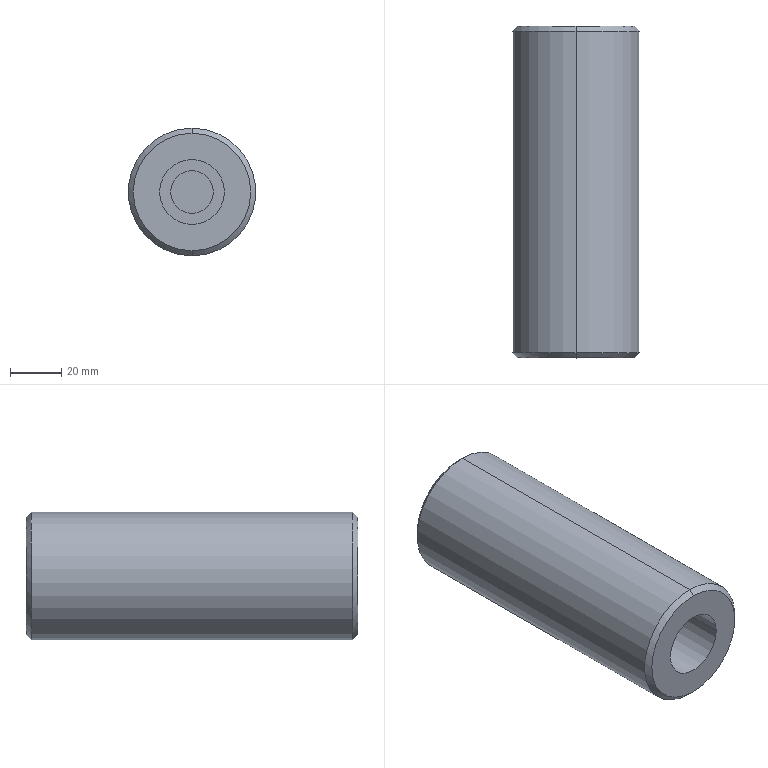Part | STEP file | 4-20.sldasm-Part-91 | 1 solid | 14 faces | box 50 x 130 x 50 mm | volume 218247 mm3 | cylinder 6 | cone 4 | plane 4 | commonest cylinder face diameters 16.667 x2 25.4 x2 50 x2
STEP:
#1=CARTESIAN_POINT('',(131.666,-614.601,200.));
#2=VERTEX_POINT('',#1);
#3=CARTESIAN_POINT('',(148.334,-614.601,200.));
#4=VERTEX_POINT('',#3);
#5=CARTESIAN_POINT('',(140.,-614.601,200.));
#6=DIRECTION('',(0.,-1.,0.));
#7=DIRECTION('',(0.,0.,-1.));
#8=AXIS2_PLACEMENT_3D('',#5,#6,#7);
#9=CIRCLE('',#8,8.334);
#10=EDGE_CURVE('',#2,#4,#9,.T.);
#11=ORIENTED_EDGE('',*,*,#10,.T.);
#12=CARTESIAN_POINT('',(148.334,-530.,200.));
#13=VERTEX_POINT('',#12);
#14=CARTESIAN_POINT('',(148.334,-632.601,200.));
#15=DIRECTION('',(0.,1.,0.));
#16=VECTOR('',#15,1000.);
#17=LINE('',#14,#16);
#18=EDGE_CURVE('',#4,#13,#17,.T.);
#19=ORIENTED_EDGE('',*,*,#18,.T.);
#20=CARTESIAN_POINT('',(131.666,-530.,200.));
#21=VERTEX_POINT('',#20);
#22=CARTESIAN_POINT('',(140.,-530.,200.));
#23=DIRECTION('',(0.,-1.,0.));
#24=DIRECTION('',(0.,0.,-1.));
#25=AXIS2_PLACEMENT_3D('',#22,#23,#24);
#26=CIRCLE('',#25,8.334);
#27=EDGE_CURVE('',#21,#13,#26,.T.);
#28=ORIENTED_EDGE('',*,*,#27,.F.);
#29=CARTESIAN_POINT('',(131.666,-632.601,200.));
#30=DIRECTION('',(0.,1.,0.));
#31=VECTOR('',#30,1000.);
#32=LINE('',#29,#31);
#33=EDGE_CURVE('',#2,#21,#32,.T.);
#34=ORIENTED_EDGE('',*,*,#33,.F.);
#35=EDGE_LOOP('',(#11,#19,#28,#34));
#36=FACE_OUTER_BOUND('',#35,.T.);
#37=CARTESIAN_POINT('',(140.,-632.601,200.));
#38=DIRECTION('',(0.,1.,0.));
#39=DIRECTION('',(-1.,0.,0.));
#40=AXIS2_PLACEMENT_3D('',#37,#38,#39);
#41=CYLINDRICAL_SURFACE('',#40,8.334);
#42=ADVANCED_FACE('',(#36),#41,.F.);
#43=CARTESIAN_POINT('',(127.3,-614.601,200.));
#44=VERTEX_POINT('',#43);
#45=CARTESIAN_POINT('',(152.7,-614.601,200.));
#46=VERTEX_POINT('',#45);
#47=CARTESIAN_POINT('',(140.,-614.601,200.));
#48=DIRECTION('',(0.,1.,0.));
#49=DIRECTION('',(0.,0.,-1.));
#50=AXIS2_PLACEMENT_3D('',#47,#48,#49);
#51=CIRCLE('',#50,12.7);
#52=EDGE_CURVE('',#44,#46,#51,.T.);
#53=ORIENTED_EDGE('',*,*,#52,.T.);
#54=CARTESIAN_POINT('',(152.7,-650.,200.));
#55=VERTEX_POINT('',#54);
#56=CARTESIAN_POINT('',(152.7,-485.,200.));
#57=DIRECTION('',(0.,-1.,0.));
#58=VECTOR('',#57,1000.);
#59=LINE('',#56,#58);
#60=EDGE_CURVE('',#46,#55,#59,.T.);
#61=ORIENTED_EDGE('',*,*,#60,.T.);
#62=CARTESIAN_POINT('',(127.3,-650.,200.));
#63=VERTEX_POINT('',#62);
#64=CARTESIAN_POINT('',(140.,-650.,200.));
#65=DIRECTION('',(0.,-1.,0.));
#66=DIRECTION('',(1.,0.,0.));
#67=AXIS2_PLACEMENT_3D('',#64,#65,#66);
#68=CIRCLE('',#67,12.7);
#69=EDGE_CURVE('',#55,#63,#68,.T.);
#70=ORIENTED_EDGE('',*,*,#69,.T.);
#71=CARTESIAN_POINT('',(127.3,-485.,200.));
#72=DIRECTION('',(0.,-1.,0.));
#73=VECTOR('',#72,1000.);
#74=LINE('',#71,#73);
#75=EDGE_CURVE('',#44,#63,#74,.T.);
#76=ORIENTED_EDGE('',*,*,#75,.F.);
#77=EDGE_LOOP('',(#53,#61,#70,#76));
#78=FACE_OUTER_BOUND('',#77,.T.);
#79=CARTESIAN_POINT('',(140.,-485.,200.));
#80=DIRECTION('',(0.,-1.,0.));
#81=DIRECTION('',(-1.,0.,0.));
#82=AXIS2_PLACEMENT_3D('',#79,#80,#81);
#83=CYLINDRICAL_SURFACE('',#82,12.7);
#84=ADVANCED_FACE('',(#78),#83,.F.);
#85=CARTESIAN_POINT('',(140.,-650.,177.));
#86=VERTEX_POINT('',#85);
#87=CARTESIAN_POINT('',(140.,-650.,223.));
#88=VERTEX_POINT('',#87);
#89=CARTESIAN_POINT('',(140.,-650.,200.));
#90=DIRECTION('',(0.,-1.,0.));
#91=DIRECTION('',(0.,0.,-1.));
#92=AXIS2_PLACEMENT_3D('',#89,#90,#91);
#93=CIRCLE('',#92,23.);
#94=EDGE_CURVE('',#86,#88,#93,.T.);
#95=ORIENTED_EDGE('',*,*,#94,.F.);
#96=CARTESIAN_POINT('',(140.,-648.,175.));
#97=VERTEX_POINT('',#96);
#98=CARTESIAN_POINT('',(140.,-650.,177.));
#99=DIRECTION('',(0.,0.7071,-0.7071));
#100=VECTOR('',#99,1000.);
#101=LINE('',#98,#100);
#102=EDGE_CURVE('',#86,#97,#101,.T.);
#103=ORIENTED_EDGE('',*,*,#102,.T.);
#104=CARTESIAN_POINT('',(140.,-648.,225.));
#105=VERTEX_POINT('',#104);
#106=CARTESIAN_POINT('',(140.,-648.,200.));
#107=DIRECTION('',(0.,1.,0.));
#108=DIRECTION('',(0.,0.,-1.));
#109=AXIS2_PLACEMENT_3D('',#106,#107,#108);
#110=CIRCLE('',#109,25.);
#111=EDGE_CURVE('',#105,#97,#110,.T.);
#112=ORIENTED_EDGE('',*,*,#111,.F.);
#113=CARTESIAN_POINT('',(140.,-650.,223.));
#114=DIRECTION('',(0.,0.7071,0.7071));
#115=VECTOR('',#114,1000.);
#116=LINE('',#113,#115);
#117=EDGE_CURVE('',#88,#105,#116,.T.);
#118=ORIENTED_EDGE('',*,*,#117,.F.);
#119=EDGE_LOOP('',(#95,#103,#112,#118));
#120=FACE_OUTER_BOUND('',#119,.T.);
#121=CARTESIAN_POINT('',(140.,-650.,200.));
#122=DIRECTION('',(0.,1.,0.));
#123=DIRECTION('',(0.,0.,1.));
#124=AXIS2_PLACEMENT_3D('',#121,#122,#123);
#125=CONICAL_SURFACE('',#124,23.,0.7854);
#126=ADVANCED_FACE('',(#120),#125,.T.);
#127=CARTESIAN_POINT('',(140.,-520.,223.));
#128=VERTEX_POINT('',#127);
#129=CARTESIAN_POINT('',(140.,-520.,177.));
#130=VERTEX_POINT('',#129);
#131=CARTESIAN_POINT('',(140.,-520.,200.));
#132=DIRECTION('',(0.,1.,0.));
#133=DIRECTION('',(0.,0.,-1.));
#134=AXIS2_PLACEMENT_3D('',#131,#132,#133);
#135=CIRCLE('',#134,23.);
#136=EDGE_CURVE('',#128,#130,#135,.T.);
#137=ORIENTED_EDGE('',*,*,#136,.F.);
#138=CARTESIAN_POINT('',(140.,-522.,225.));
#139=VERTEX_POINT('',#138);
#140=CARTESIAN_POINT('',(140.,-522.,225.));
#141=DIRECTION('',(0.,-0.7071,0.7071));
#142=VECTOR('',#141,1000.);
#143=LINE('',#140,#142);
#144=EDGE_CURVE('',#128,#139,#143,.T.);
#145=ORIENTED_EDGE('',*,*,#144,.T.);
#146=CARTESIAN_POINT('',(140.,-522.,175.));
#147=VERTEX_POINT('',#146);
#148=CARTESIAN_POINT('',(140.,-522.,200.));
#149=DIRECTION('',(0.,-1.,0.));
#150=DIRECTION('',(0.,0.,-1.));
#151=AXIS2_PLACEMENT_3D('',#148,#149,#150);
#152=CIRCLE('',#151,25.);
#153=EDGE_CURVE('',#147,#139,#152,.T.);
#154=ORIENTED_EDGE('',*,*,#153,.F.);
#155=CARTESIAN_POINT('',(140.,-522.,175.));
#156=DIRECTION('',(0.,-0.7071,-0.7071));
#157=VECTOR('',#156,1000.);
#158=LINE('',#155,#157);
#159=EDGE_CURVE('',#130,#147,#158,.T.);
#160=ORIENTED_EDGE('',*,*,#159,.F.);
#161=EDGE_LOOP('',(#137,#145,#154,#160));
#162=FACE_OUTER_BOUND('',#161,.T.);
#163=CARTESIAN_POINT('',(140.,-522.,200.));
#164=DIRECTION('',(0.,-1.,0.));
#165=DIRECTION('',(0.,0.,-1.));
#166=AXIS2_PLACEMENT_3D('',#163,#164,#165);
#167=CONICAL_SURFACE('',#166,25.,0.7854);
#168=ADVANCED_FACE('',(#162),#167,.T.);
#169=ORIENTED_EDGE('',*,*,#111,.T.);
#170=CARTESIAN_POINT('',(140.,-570.,175.));
#171=DIRECTION('',(0.,1.,0.));
#172=VECTOR('',#171,1000.);
#173=LINE('',#170,#172);
#174=EDGE_CURVE('',#97,#147,#173,.T.);
#175=ORIENTED_EDGE('',*,*,#174,.T.);
#176=ORIENTED_EDGE('',*,*,#153,.T.);
#177=CARTESIAN_POINT('',(140.,-570.,225.));
#178=DIRECTION('',(0.,1.,0.));
#179=VECTOR('',#178,1000.);
#180=LINE('',#177,#179);
#181=EDGE_CURVE('',#105,#139,#180,.T.);
#182=ORIENTED_EDGE('',*,*,#181,.F.);
#183=EDGE_LOOP('',(#169,#175,#176,#182));
#184=FACE_OUTER_BOUND('',#183,.T.);
#185=CARTESIAN_POINT('',(140.,-570.,200.));
#186=DIRECTION('',(0.,1.,0.));
#187=DIRECTION('',(0.,0.,1.));
#188=AXIS2_PLACEMENT_3D('',#185,#186,#187);
#189=CYLINDRICAL_SURFACE('',#188,25.);
#190=ADVANCED_FACE('',(#184),#189,.T.);
#191=ORIENTED_EDGE('',*,*,#174,.F.);
#192=CARTESIAN_POINT('',(140.,-648.,200.));
#193=DIRECTION('',(0.,1.,0.));
#194=DIRECTION('',(0.,0.,-1.));
#195=AXIS2_PLACEMENT_3D('',#192,#193,#194);
#196=CIRCLE('',#195,25.);
#197=EDGE_CURVE('',#97,#105,#196,.T.);
#198=ORIENTED_EDGE('',*,*,#197,.T.);
#199=ORIENTED_EDGE('',*,*,#181,.T.);
#200=CARTESIAN_POINT('',(140.,-522.,200.));
#201=DIRECTION('',(0.,-1.,0.));
#202=DIRECTION('',(0.,0.,-1.));
#203=AXIS2_PLACEMENT_3D('',#200,#201,#202);
#204=CIRCLE('',#203,25.);
#205=EDGE_CURVE('',#139,#147,#204,.T.);
#206=ORIENTED_EDGE('',*,*,#205,.T.);
#207=EDGE_LOOP('',(#191,#198,#199,#206));
#208=FACE_OUTER_BOUND('',#207,.T.);
#209=CARTESIAN_POINT('',(140.,-570.,200.));
#210=DIRECTION('',(0.,1.,0.));
#211=DIRECTION('',(0.,0.,1.));
#212=AXIS2_PLACEMENT_3D('',#209,#210,#211);
#213=CYLINDRICAL_SURFACE('',#212,25.);
#214=ADVANCED_FACE('',(#208),#213,.T.);
#215=CARTESIAN_POINT('',(140.,-650.,200.));
#216=DIRECTION('',(0.,-1.,0.));
#217=DIRECTION('',(1.,0.,0.));
#218=AXIS2_PLACEMENT_3D('',#215,#216,#217);
#219=CIRCLE('',#218,12.7);
#220=EDGE_CURVE('',#63,#55,#219,.T.);
#221=ORIENTED_EDGE('',*,*,#220,.F.);
#222=ORIENTED_EDGE('',*,*,#69,.F.);
#223=EDGE_LOOP('',(#221,#222));
#224=FACE_BOUND('',#223,.T.);
#225=CARTESIAN_POINT('',(140.,-650.,200.));
#226=DIRECTION('',(0.,-1.,0.));
#227=DIRECTION('',(0.,0.,-1.));
#228=AXIS2_PLACEMENT_3D('',#225,#226,#227);
#229=CIRCLE('',#228,23.);
#230=EDGE_CURVE('',#88,#86,#229,.T.);
#231=ORIENTED_EDGE('',*,*,#230,.T.);
#232=ORIENTED_EDGE('',*,*,#94,.T.);
#233=EDGE_LOOP('',(#231,#232));
#234=FACE_OUTER_BOUND('',#233,.T.);
#235=CARTESIAN_POINT('',(112.5,-650.,719.));
#236=DIRECTION('',(0.,-1.,0.));
#237=DIRECTION('',(0.,0.,-1.));
#238=AXIS2_PLACEMENT_3D('',#235,#236,#237);
#239=PLANE('',#238);
#240=ADVANCED_FACE('',(#224,#234),#239,.T.);
#241=CARTESIAN_POINT('',(140.,-520.,200.));
#242=DIRECTION('',(0.,1.,0.));
#243=DIRECTION('',(0.,0.,-1.));
#244=AXIS2_PLACEMENT_3D('',#241,#242,#243);
#245=CIRCLE('',#244,23.);
#246=EDGE_CURVE('',#130,#128,#245,.T.);
#247=ORIENTED_EDGE('',*,*,#246,.T.);
#248=ORIENTED_EDGE('',*,*,#136,.T.);
#249=EDGE_LOOP('',(#247,#248));
#250=FACE_OUTER_BOUND('',#249,.T.);
#251=CARTESIAN_POINT('',(140.,-520.,200.));
#252=DIRECTION('',(0.,-1.,0.));
#253=DIRECTION('',(0.,0.,-1.));
#254=AXIS2_PLACEMENT_3D('',#251,#252,#253);
#255=PLANE('',#254);
#256=ADVANCED_FACE('',(#250),#255,.F.);
#257=ORIENTED_EDGE('',*,*,#144,.F.);
#258=ORIENTED_EDGE('',*,*,#246,.F.);
#259=ORIENTED_EDGE('',*,*,#159,.T.);
#260=ORIENTED_EDGE('',*,*,#205,.F.);
#261=EDGE_LOOP('',(#257,#258,#259,#260));
#262=FACE_OUTER_BOUND('',#261,.T.);
#263=CARTESIAN_POINT('',(140.,-522.,200.));
#264=DIRECTION('',(0.,-1.,0.));
#265=DIRECTION('',(0.,0.,-1.));
#266=AXIS2_PLACEMENT_3D('',#263,#264,#265);
#267=CONICAL_SURFACE('',#266,25.,0.7854);
#268=ADVANCED_FACE('',(#262),#267,.T.);
#269=ORIENTED_EDGE('',*,*,#102,.F.);
#270=ORIENTED_EDGE('',*,*,#230,.F.);
#271=ORIENTED_EDGE('',*,*,#117,.T.);
#272=ORIENTED_EDGE('',*,*,#197,.F.);
#273=EDGE_LOOP('',(#269,#270,#271,#272));
#274=FACE_OUTER_BOUND('',#273,.T.);
#275=CARTESIAN_POINT('',(140.,-650.,200.));
#276=DIRECTION('',(0.,1.,0.));
#277=DIRECTION('',(0.,0.,1.));
#278=AXIS2_PLACEMENT_3D('',#275,#276,#277);
#279=CONICAL_SURFACE('',#278,23.,0.7854);
#280=ADVANCED_FACE('',(#274),#279,.T.);
#281=ORIENTED_EDGE('',*,*,#60,.F.);
#282=CARTESIAN_POINT('',(140.,-614.601,200.));
#283=DIRECTION('',(0.,1.,0.));
#284=DIRECTION('',(0.,0.,-1.));
#285=AXIS2_PLACEMENT_3D('',#282,#283,#284);
#286=CIRCLE('',#285,12.7);
#287=EDGE_CURVE('',#46,#44,#286,.T.);
#288=ORIENTED_EDGE('',*,*,#287,.T.);
#289=ORIENTED_EDGE('',*,*,#75,.T.);
#290=ORIENTED_EDGE('',*,*,#220,.T.);
#291=EDGE_LOOP('',(#281,#288,#289,#290));
#292=FACE_OUTER_BOUND('',#291,.T.);
#293=CARTESIAN_POINT('',(140.,-485.,200.));
#294=DIRECTION('',(0.,-1.,0.));
#295=DIRECTION('',(-1.,0.,0.));
#296=AXIS2_PLACEMENT_3D('',#293,#294,#295);
#297=CYLINDRICAL_SURFACE('',#296,12.7);
#298=ADVANCED_FACE('',(#292),#297,.F.);
#299=ORIENTED_EDGE('',*,*,#18,.F.);
#300=CARTESIAN_POINT('',(140.,-614.601,200.));
#301=DIRECTION('',(0.,-1.,0.));
#302=DIRECTION('',(0.,0.,-1.));
#303=AXIS2_PLACEMENT_3D('',#300,#301,#302);
#304=CIRCLE('',#303,8.334);
#305=EDGE_CURVE('',#4,#2,#304,.T.);
#306=ORIENTED_EDGE('',*,*,#305,.T.);
#307=ORIENTED_EDGE('',*,*,#33,.T.);
#308=CARTESIAN_POINT('',(140.,-530.,200.));
#309=DIRECTION('',(0.,-1.,0.));
#310=DIRECTION('',(0.,0.,-1.));
#311=AXIS2_PLACEMENT_3D('',#308,#309,#310);
#312=CIRCLE('',#311,8.334);
#313=EDGE_CURVE('',#13,#21,#312,.T.);
#314=ORIENTED_EDGE('',*,*,#313,.F.);
#315=EDGE_LOOP('',(#299,#306,#307,#314));
#316=FACE_OUTER_BOUND('',#315,.T.);
#317=CARTESIAN_POINT('',(140.,-632.601,200.));
#318=DIRECTION('',(0.,1.,0.));
#319=DIRECTION('',(-1.,0.,0.));
#320=AXIS2_PLACEMENT_3D('',#317,#318,#319);
#321=CYLINDRICAL_SURFACE('',#320,8.334);
#322=ADVANCED_FACE('',(#316),#321,.F.);
#323=ORIENTED_EDGE('',*,*,#10,.F.);
#324=ORIENTED_EDGE('',*,*,#305,.F.);
#325=EDGE_LOOP('',(#323,#324));
#326=FACE_BOUND('',#325,.T.);
#327=ORIENTED_EDGE('',*,*,#52,.F.);
#328=ORIENTED_EDGE('',*,*,#287,.F.);
#329=EDGE_LOOP('',(#327,#328));
#330=FACE_OUTER_BOUND('',#329,.T.);
#331=CARTESIAN_POINT('',(140.,-614.601,200.));
#332=DIRECTION('',(0.,1.,0.));
#333=DIRECTION('',(-1.,0.,0.));
#334=AXIS2_PLACEMENT_3D('',#331,#332,#333);
#335=PLANE('',#334);
#336=ADVANCED_FACE('',(#326,#330),#335,.F.);
#337=ORIENTED_EDGE('',*,*,#27,.T.);
#338=ORIENTED_EDGE('',*,*,#313,.T.);
#339=EDGE_LOOP('',(#337,#338));
#340=FACE_OUTER_BOUND('',#339,.T.);
#341=CARTESIAN_POINT('',(154.5,-530.,-422.));
#342=DIRECTION('',(0.,1.,0.));
#343=DIRECTION('',(1.,0.,0.));
#344=AXIS2_PLACEMENT_3D('',#341,#342,#343);
#345=PLANE('',#344);
#346=ADVANCED_FACE('',(#340),#345,.F.);
#347=CLOSED_SHELL('',(#42,#84,#126,#168,#190,#214,#240,#256,#268,#280,#298,#322,#336,#346));
#348=MANIFOLD_SOLID_BREP('',#347);
#349=CARTESIAN_POINT('',(0.,0.,0.));
#350=DIRECTION('',(0.,0.,1.));
#351=DIRECTION('',(1.,0.,0.));
#352=AXIS2_PLACEMENT_3D('',#349,#350,#351);
#353=(LENGTH_UNIT()NAMED_UNIT(*)SI_UNIT(.MILLI.,.METRE.));
#354=UNCERTAINTY_MEASURE_WITH_UNIT(LENGTH_MEASURE(0.00001),#353,'','');
#355=(NAMED_UNIT(*)PLANE_ANGLE_UNIT()SI_UNIT($,.RADIAN.));
#356=(NAMED_UNIT(*)SI_UNIT($,.STERADIAN.)SOLID_ANGLE_UNIT());
#357=(GEOMETRIC_REPRESENTATION_CONTEXT(3)GLOBAL_UNCERTAINTY_ASSIGNED_CONTEXT((#354))GLOBAL_UNIT_ASSIGNED_CONTEXT((#353,#355,#356))REPRESENTATION_CONTEXT('',''));
#358=ADVANCED_BREP_SHAPE_REPRESENTATION('',(#348,#352),#357);